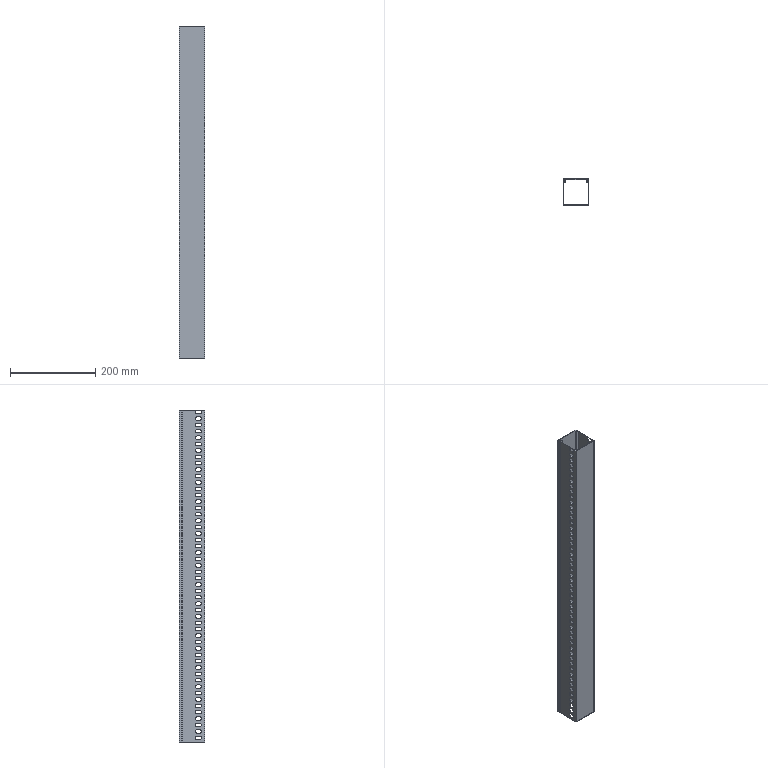Part | SolidWorks | features BaseBody 1 | 1 solid | 442 faces | box 60 x 60 x 780 mm | volume 189460 mm3 | plane 234 | cylinder 208 | commonest cylinder face diameters 8 x208